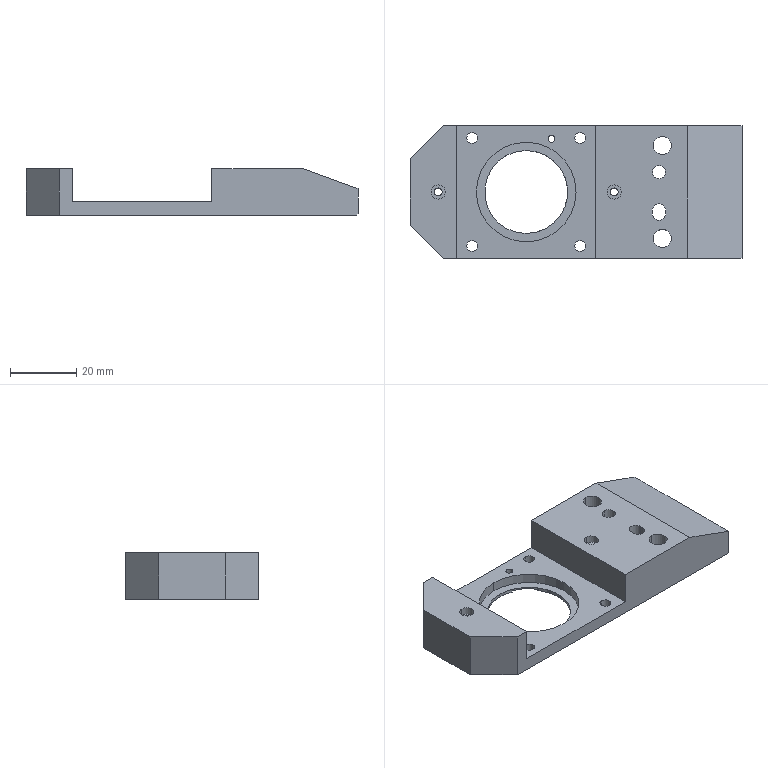NC program | NX | posted with a generic post | part box 100 x 40 x 14 mm
Lines 19 to 1361 of 15435:
(ADAPTIVE_MILLING_COPY , TOOL : D10)
N36 T04 M6
N38 G54
N40 G17 G0 G90 X-60.658 Y-0.012 S4000 M3
N42 G43 Z30. H4
N44 Z-13.
N46 G94 G1 Z-14. F1000.
N48 X-59.988 Y-0.372 F2200.
N50 X-59.306 Y-0.709
N52 G3 X-58.012 Y-0.012 R1.014
N54 X-57.807 Y4.262 R25.796
N56 G1 X-57.804 Y5.087
N58 X-57.802 Y6.337
N60 X-57.801 Y8.662
N62 X-57.8 Y21.587
N64 Y21.687
N66 X-57.797 Y21.787
N68 G2 X-54.247 Y26.731 R5.868
N70 X-49.332 Y27.731 R12.663
N72 X-41.858 Y27.797 R436.949
N74 G1 X-17.558
N76 X51.642
N78 X51.742 Y27.795
N80 X51.842 Y27.791
N82 X51.917 Y27.787
N84 X51.992 Y27.782
N86 G2 X56.775 Y24.149 R5.928
N88 X57.741 Y19.049 R13.335
N90 X57.796 Y11.775 R571.146
N92 G1 Y-21.6
N94 X57.795 Y-21.7
N96 X57.793 Y-21.775
N98 X57.79 Y-21.85
N100 X57.784 Y-21.95
N102 X57.778 Y-22.025
N104 G2 X54.072 Y-26.81 R5.956
N106 X49.165 Y-27.738 R13.286
N108 X37.666 Y-27.797 R661.267
N110 G1 X-51.634
N112 X-51.734 Y-27.795
N114 X-51.834 Y-27.792
N116 X-51.909 Y-27.787
N118 X-51.984 Y-27.782
N120 X-52.084 Y-27.773
N122 G2 X-56.813 Y-24.064 R5.968
N124 X-57.741 Y-19.031 R13.527
N126 X-57.764 Y-0.657 R809.741
N128 G3 X-57.604 Y8.715 R170.554
N130 G2 X-57.575 Y20.839 R747.675
N132 X-53.065 Y26.591 R6.941
N134 X-47.75 Y27.529 R15.579
N136 X-38.776 Y27.595 R512.073
N138 G1 X-9.076
N140 X-8.226 Y27.596
N142 X-7.826
N144 X-7.476
N146 X-7.201
N148 X-6.801 Y27.597
N150 X-5.826
N152 X-4.526
N154 X-4.051
N156 X-3.701
N158 X-3.376
N160 X-3.026
N162 X-2.701
N164 X-2.351
N166 X-2.026
N168 X-1.676
N170 X-1.351
N172 X-1.001
N174 X-0.651
N176 X-0.326
N178 X0.599
N180 X1.524
N182 X2.699
N184 X3.499
N186 X4.974
N188 X5.399
N190 X6.424
N192 X7.224
N194 X7.874
N196 X9.024
N198 X9.849
N200 X10.749
N202 X12.074
N204 X12.399
N206 X12.824
N208 X13.449
N210 X14.049
N212 X14.674
N214 X15.274
N216 X15.899
N218 X17.099
N220 X17.924
N222 X18.249
N224 X18.674
N226 X21.174
N228 X22.599
N230 X23.749
N232 X24.399
N234 X25.024
N236 X25.824
N238 X27.249 Y27.598
N240 X27.924 Y27.597
N242 X28.724
N244 X29.124
N246 X30.474
N248 X31.174
N250 X31.474
N252 X31.799
N254 X32.099
N256 X32.924
N258 X33.224
N260 X33.524
N262 X33.849
N264 X34.199
N266 X34.499
N268 X35.324
N270 X35.649
N272 X36.074
N274 X36.699
N276 X37.899
N278 X38.724
N280 X39.049
N282 X39.474
N284 X40.799 Y27.598
N286 X41.874 Y27.597
N288 X43.199
N290 X43.524
N292 X43.849
N294 X44.174
N296 X45.274 Y27.598
N298 X45.599 Y27.597
N300 X46.424
N302 X46.774
N304 X47.124
N306 X47.449
N308 X47.799
N310 X48.149
N312 X48.499
N314 X48.824
N316 X49.174
N318 X49.524
N320 X49.874
N322 X50.249
N324 X50.374 Y27.595
N326 X50.474 Y27.593
N328 X50.549 Y27.59
N330 X50.649 Y27.584
N332 X50.723 Y27.579
N334 X50.823 Y27.572
N336 G2 X56.565 Y23.122 R6.923
N338 X57.528 Y17.737 R15.471
N340 X57.594 Y8.263 R533.615
N342 G1 Y-20.262
N344 X57.593 Y-20.362
N346 X57.59 Y-20.462
N348 X57.586 Y-20.562
N350 X57.581 Y-20.662
N352 X57.574 Y-20.762
N354 G2 X53.061 Y-26.59 R6.93
N356 X47.671 Y-27.531 R15.729
N358 X37.197 Y-27.595 R619.863
N360 G1 X-50.253
N362 X-50.378 Y-27.593
N364 X-50.478 Y-27.59
N366 X-50.578 Y-27.586
N368 X-50.678 Y-27.581
N370 X-50.777 Y-27.573
N372 G2 X-56.576 Y-23.093 R6.924
N374 X-57.534 Y-17.556 R15.875
N376 X-57.552 Y-0.857 R593.714
N378 G3 X-57.405 Y10.841 R287.782
N380 G2 X-57.367 Y19.915 R332.032
N382 X-52.272 Y26.382 R7.62
N384 X-46.402 Y27.333 R17.997
N386 X-31.028 Y27.393 R794.051
N388 G1 X-10.478
N390 X-10.153 Y27.394
N392 X-9.853
N394 X-9.478 Y27.395
N396 X-8.753
N398 X-8.178
N400 X-7.628 Y27.396
N402 X-7.278
N404 X-6.928
N406 X-6.128
N408 X-5.353 Y27.397
N410 X-5.028
N412 X-4.603
N414 X-4.053
N416 X-3.553
N418 X-2.953
N420 X-2.653
N422 X-2.353
N424 X-1.978
N426 X-1.578
N428 X-0.778
N430 X-0.078
N432 X1.297
N434 X2.897 Y27.398
N436 X3.547 Y27.397
N438 X4.022
N440 X4.322
N442 X4.622
N444 X6.547
N446 X7.422
N448 X7.972
N450 X8.497
N452 X8.822
N454 X9.197
N456 X10.197
N458 X11.222
N460 X12.047
N462 X12.722
N464 X13.272
N466 X14.072
N468 X14.397
N470 X15.397
N472 X16.172
N474 X16.672
N476 X17.272
N478 X18.372
N480 X18.722
N482 X19.672
N484 X19.997
N486 X20.397
N488 X21.047
N490 X21.472
N492 X21.872
N494 X22.647
N496 X23.047
N498 X23.622
N500 X25.147
N502 X26.472
N504 X27.022
N506 X27.347
N508 X27.672
N510 X27.972
N512 X28.347
N514 X30.472
N516 X31.297
N518 X32.322
N520 X32.822
N522 X33.222
N524 X34.022
N526 X34.422
N528 X34.947
N530 G2 X49.871 Y27.364 R852.398
N532 X56.365 Y22.307 R7.605
N534 X57.328 Y16.49 R17.652
N536 X57.392 Y6.341 R626.425
N538 G1 Y-19.034
N540 X57.391 Y-19.184
N542 X57.388 Y-19.309
N544 X57.384 Y-19.459
N546 X57.379 Y-19.584
N548 X57.372 Y-19.709
N550 G2 X52.293 Y-26.371 R7.602
N552 X46.5 Y-27.328 R17.677
N554 X35.426 Y-27.393 R648.625
N556 G1 X-49.024
N558 X-49.199 Y-27.391
N560 X-49.349 Y-27.388
N562 X-49.474 Y-27.384
N564 X-49.599 Y-27.379
N566 X-49.724 Y-27.371
N568 G2 X-56.366 Y-22.303 R7.598
N570 X-57.32 Y-16.685 R17.277
N572 X-57.224 Y4.487 R468.954
N574 X-57.172 Y18.961 R932.099
N576 X-51.572 Y26.18 R8.162
N578 X-45.672 Y27.121 R19.16
N580 X-28.373 Y27.191 R845.532
N582 G1 X-11.873
N584 X-11.498 Y27.192
N586 X-11.123
N588 X-10.723 Y27.193
N590 X-10.273
N592 X-9.948 Y27.194
N594 X-9.548
N596 X-8.973 Y27.195
N598 X-8.648
N600 X-8.298
N602 X-7.998
N604 X-7.173 Y27.196
N606 X-6.773
N608 X-5.948
N610 X-5.423 Y27.197
N612 X-4.473
N614 X-3.023
N616 X-2.748
N618 X-2.473
N620 X-2.173
N622 X-1.798
N624 X-1.248
N626 X-0.373
N628 X0.977 Y27.198
N630 X1.252 Y27.197
N632 X1.552 Y27.198
N634 X2.377 Y27.197
N636 X2.802 Y27.198
N638 X3.402
N640 X4.552
N642 X5.002 Y27.197
N644 X5.377
N646 X5.677
N648 X6.677
N650 X7.152
N652 X7.477
N654 X7.877
N656 X8.627
N658 X8.927
N660 X9.627
N662 X10.152
N664 X10.452
N666 X11.302
N668 X11.977
N670 X12.477
N672 X13.327
N674 X13.652 Y27.198
N676 X14.027 Y27.197
N678 X14.552
N680 X15.052 Y27.198
N682 X17.102 Y27.197
N684 X17.677
N686 X17.977
N688 X18.327
N690 X18.627
N692 X18.927
N694 X19.302
N696 X19.627
N698 X20.727
N700 X21.402
N702 X22.027
N704 X22.627
N706 X23.702
N708 X24.102
N710 X24.852
N712 X25.877 Y27.198
N714 X26.677 Y27.197
N716 X27.202
N718 X27.527
N720 X28.652
N722 X29.952
N724 X30.552
N726 X30.852
N728 X31.427
N730 X32.277
N732 X32.652
N734 X32.977
N736 X33.252
N738 X33.552
N740 X33.927
N742 X34.177
N744 X34.502
N746 X34.852
N748 X35.777
N750 X36.627
N752 X36.977
N754 X37.277
N756 X37.702
N758 G2 X49.002 Y27.161 R605.97
N760 X56.159 Y21.621 R8.144
N762 X57.122 Y15.575 R19.209
N764 X57.19 Y5.55 R621.552
N766 G1 Y-17.95
N768 X57.188 Y-18.15
N770 X57.186 Y-18.325
N772 X57.182 Y-18.5
N774 X57.176 Y-18.649
N776 X57.169 Y-18.799
N778 G2 X51.667 Y-26.142 R8.138
N780 X45.649 Y-27.12 R18.936
N782 X29.05 Y-27.191 R817.893
N784 G1 X-8.375
N786 X-9.225 Y-27.192
N788 X-9.625
N790 X-10.1
N792 X-10.525
N794 X-10.875
N796 X-11.2 Y-27.193
N798 X-12.125
N800 X-12.975
N802 X-13.275
N804 X-13.575
N806 X-15.125
N808 X-15.825
N810 X-17.
N812 X-17.7
N814 X-18.875
N816 X-19.425
N818 X-19.775
N820 X-20.1
N822 X-21.2
N824 X-21.525
N826 X-21.85
N828 X-22.675
N830 X-23.65
N832 X-24.275
N834 X-25.6
N836 X-26.2
N838 X-26.525
N840 X-26.825
N842 X-27.65
N844 X-28.45
N846 X-29.625
N848 X-30.275
N850 X-30.875
N852 X-31.5
N854 X-32.1
N856 X-32.725
N858 X-33.325
N860 X-33.95
N862 X-34.55
N864 X-35.175
N866 X-35.775
N868 X-36.4
N870 X-37.
N872 X-37.625
N874 X-38.225
N876 X-38.85
N878 X-39.45
N880 X-40.075
N882 X-40.675
N884 X-41.3
N886 G2 X-49.174 Y-27.144 R190.539
N888 X-56.123 Y-21.714 R8.121
N890 X-57.115 Y-15.774 R18.568
N892 X-57.026 Y4.774 R495.094
N894 X-56.966 Y18.248 R708.359
N896 X-51.062 Y25.935 R8.596
N898 X-44.966 Y26.912 R20.074
N900 X-33.916 Y26.989 R534.348
N902 G1 X-13.291
N904 X-12.891 Y26.99
N906 X-12.591
N908 X-12.166 Y26.991
N910 X-11.216 Y26.992
N912 X-10.566 Y26.993
N914 X-10.016
N916 X-9.216 Y26.994
N918 X-8.366 Y26.995
N920 X-7.216 Y26.996
N922 X-6.666
N924 X-6.266
N926 X-5.816
N928 X-4.516
N930 X-3.716 Y26.997
N932 X-2.866
N934 X-2.566
N936 X-2.291
N938 X-1.966
N940 X-1.641
N942 X-0.741
N944 X-0.116
N946 X0.309
N948 X1.109
N950 X2.034
N952 X2.609
N954 X3.209 Y26.998
N956 X3.609 Y26.997
N958 X4.009 Y26.998
N960 X4.309 Y26.997
N962 X4.684
N964 X5.234
N966 X5.534
N968 X6.159
N970 X6.959
N972 X7.359
N974 X7.959
N976 X8.484
N978 X8.834
N980 X10.234
N982 X10.534
N984 X10.834
N986 X11.734
N988 X12.259
N990 X12.609
N992 X13.009
N994 X13.309
N996 X13.709 Y26.998
N998 X14.659 Y26.997
N1000 X16.384
N1002 X16.684
N1004 X16.984
N1006 X17.409
N1008 X18.084
N1010 X19.709
N1012 X20.634
N1014 X21.259
N1016 X21.784
N1018 X22.709
N1020 X23.859
N1022 X24.434 Y26.998
N1024 X24.909 Y26.997
N1026 X26.509
N1028 X27.409
N1030 X28.659
N1032 X29.509
N1034 X29.884
N1036 X30.459
N1038 X30.959
N1040 X31.259
N1042 X31.609
N1044 X32.009
N1046 X32.534
N1048 X32.909
N1050 X33.184
N1052 X33.484
N1054 X34.359
N1056 G2 X48.233 Y26.958 R698.776
N1058 X55.939 Y21.045 R8.594
N1060 X56.913 Y14.873 R20.196
N1062 X56.988 Y1.748 R627.827
N1064 G1 Y-16.977
N1066 X56.987 Y-17.152
N1068 X56.985 Y-17.352
N1070 X56.982 Y-17.527
N1072 X56.977 Y-17.702
N1074 X56.971 Y-17.877
N1076 G2 X50.93 Y-25.98 R8.63
N1078 X44.576 Y-26.924 R21.193
N1080 X33.476 Y-26.989 R651.446
N1082 G1 X-6.974
N1084 X-7.299 Y-26.99
N1086 X-7.599
N1088 X-7.974
N1090 X-8.874 Y-26.991
N1092 X-9.174
N1094 X-9.549
N1096 X-10.124 Y-26.992
N1098 X-10.424
N1100 X-10.799
N1102 X-11.349
N1104 X-11.674
N1106 X-12.224 Y-26.993
N1108 X-12.524 Y-26.992
N1110 X-13.474 Y-26.993
N1112 X-13.749
N1114 X-15.549
N1116 X-16.799
N1118 X-18.199
N1120 X-20.524
N1122 X-21.074
N1124 X-21.924
N1126 X-22.499
N1128 X-22.799
N1130 X-23.349
N1132 X-23.699
N1134 X-24.574
N1136 X-24.874
N1138 X-25.174
N1140 X-25.599
N1142 X-26.074
N1144 X-26.849
N1146 X-27.124
N1148 X-27.399
N1150 X-27.699
N1152 X-28.674
N1154 X-29.524
N1156 X-30.074
N1158 X-30.924
N1160 X-31.249
N1162 X-31.674
N1164 X-32.274
N1166 X-32.824
N1168 X-33.524
N1170 X-33.974
N1172 X-34.274
N1174 X-34.624
N1176 X-35.074
N1178 X-35.599
N1180 X-36.274
N1182 X-36.749
N1184 X-37.049
N1186 X-37.349
N1188 X-38.249
N1190 X-38.624
N1192 X-39.349
N1194 X-39.824
N1196 X-40.124
N1198 X-40.499
N1200 X-41.349
N1202 X-41.649
N1204 G2 X-48.597 Y-26.924 R116.253
N1206 X-55.944 Y-21.028 R8.585
N1208 X-56.92 Y-14.705 R20.626
N1210 X-56.826 Y5.168 R529.552
N1212 X-56.764 Y17.542 R590.002
N1214 X-50.503 Y25.728 R8.999
N1216 X-44.004 Y26.715 R21.688
N1218 X-34.404 Y26.786 R610.822
N1220 G1 X-20.479 Y26.787
N1222 X-14.704
N1224 X-14.279 Y26.788
N1226 X-13.979
N1228 X-13.629 Y26.789
N1230 X-13.304
N1232 X-12.929
N1234 X-12.304 Y26.79
N1236 X-11.604 Y26.791
N1238 X-9.829 Y26.794
N1240 X-8.904
N1242 X-8.504
N1244 X-8.004 Y26.795
N1246 X-7.204
N1248 X-6.879
N1250 X-6.054 Y26.796
N1252 X-4.879 Y26.797
N1254 X-4.554
N1256 X-3.929
N1258 X-3.529
N1260 X-2.904
N1262 X-2.429
N1264 X-1.554
N1266 X-1.179
N1268 X-0.879
N1270 X0.121
N1272 X0.946
N1274 X1.246
N1276 X1.871 Y26.798
N1278 X2.221 Y26.797
N1280 X2.621 Y26.798
N1282 X2.921 Y26.797
N1284 X3.321
N1286 X3.596
N1288 X3.971
N1290 X4.471
N1292 X4.771
N1294 X5.071
N1296 X5.371
N1298 X5.921
N1300 X6.221
N1302 X6.921
N1304 X7.446
N1306 X8.421
N1308 X9.246
N1310 X9.521
N1312 X9.821
N1314 X10.796
N1316 X11.746
N1318 X12.296
N1320 X12.596
N1322 X12.921
N1324 X13.296
N1326 X13.821
N1328 X14.696
N1330 X15.046
N1332 X15.746
N1334 X16.246
N1336 X16.571
N1338 X16.946
N1340 X17.246
N1342 X17.571
N1344 X19.021
N1346 X20.196
N1348 X21.646
N1350 X21.946
N1352 X22.771
N1354 X23.071
N1356 X23.396
N1358 X23.746
N1360 X24.146
N1362 X25.471
N1364 X26.321
N1366 X27.496
N1368 X27.821
N1370 X28.221
N1372 X28.696
N1374 X28.996
N1376 X29.346
N1378 X29.771
N1380 X30.396
N1382 X30.971
N1384 X31.521
N1386 X31.871
N1388 X32.421
N1390 G2 X47.47 Y26.759 R837.178
N1392 X55.746 Y20.445 R9.005
N1394 X56.71 Y14.067 R21.68
N1396 X56.786 Y0.243 R684.127
N1398 G1 X56.785 Y-16.107
N1400 X56.784 Y-16.357
N1402 X56.782 Y-16.582
N1404 X56.778 Y-16.807
N1406 X56.773 Y-16.982
N1408 X56.766 Y-17.182
N1410 G2 X50.477 Y-25.734 R9.013
N1412 X44.301 Y-26.702 R21.031
N1414 X34.077 Y-26.786 R443.88
N1416 G1 X16.577 Y-26.787
N1418 X-5.573
N1420 X-5.923 Y-26.788
N1422 X-6.223
N1424 X-6.573 Y-26.789
N1426 X-6.898
N1428 X-7.223
N1430 X-7.548
N1432 X-7.973 Y-26.79
N1434 X-8.548
N1436 X-9.423 Y-26.791
N1438 X-10.223
N1440 X-10.523
N1442 X-10.923 Y-26.792
N1444 X-11.748
N1446 X-12.098
N1448 X-12.398
N1450 X-12.698
N1452 X-13.523 Y-26.793
N1454 X-14.848
N1456 X-16.323
N1458 X-17.098
N1460 X-17.398
N1462 X-17.698
N1464 X-18.723
N1466 X-20.298
N1468 X-21.123
N1470 X-21.498
N1472 X-22.073
N1474 X-23.173
N1476 X-23.648
N1478 X-24.448
N1480 X-25.548
N1482 X-25.823
N1484 X-26.123
N1486 X-26.448
N1488 X-27.048
N1490 X-27.898
N1492 X-28.423
N1494 X-28.723
N1496 X-29.573
N1498 X-29.998
N1500 X-30.873
N1502 X-31.123
N1504 X-31.423
N1506 X-31.848
N1508 X-32.423
N1510 X-33.073
N1512 X-33.548
N1514 X-33.898
N1516 X-34.198
N1518 X-34.548
N1520 X-35.398
N1522 X-35.773
N1524 X-36.623
N1526 X-36.898
N1528 X-37.223
N1530 X-37.648
N1532 X-38.248
N1534 X-38.823
N1536 X-40.048
N1538 G2 X-47.797 Y-26.731 R166.798
N1540 X-55.721 Y-20.51 R8.973
N1542 X-56.713 Y-14.012 R21.589
N1544 X-56.631 Y5.186 R521.074
N1546 X-56.557 Y16.96 R462.345
N1548 X-50.06 Y25.493 R9.334
N1550 X-43.538 Y26.503 R22.039
N1552 X-32.864 Y26.584 R503.238
N1554 G1 X-16.114 Y26.585
N1556 X-15.689 Y26.586
N1558 X-15.339
N1560 X-15.014 Y26.587
N1562 X-14.714
N1564 X-14.314
N1566 X-13.739 Y26.588
N1568 X-13.464 Y26.589
N1570 X-13.139
N1572 X-12.764 Y26.59
N1574 X-12.464
N1576 X-12.164
N1578 X-11.314 Y26.592
N1580 X-10.789
N1582 X-10.139 Y26.593
N1584 X-9.239
N1586 X-8.114 Y26.594
N1588 X-6.614 Y26.595
N1590 X-6.264 Y26.596
N1592 X-5.939
N1594 X-5.539
N1596 X-4.914
N1598 X-4.289
N1600 X-3.789
N1602 X-3.514
N1604 X-3.189 Y26.597
N1606 X-2.814
N1608 X-2.564
N1610 X-2.264
N1612 X-1.889
N1614 X-1.439
N1616 X-0.964
N1618 X-0.589
N1620 X0.361 Y26.598
N1622 X0.886 Y26.597
N1624 X1.161 Y26.598
N1626 X1.536 Y26.597
N1628 X1.886
N1630 X2.236
N1632 X2.536
N1634 X2.911
N1636 X3.461
N1638 X3.836
N1640 X4.311
N1642 X4.636
N1644 X5.186
N1646 X5.511
N1648 X6.161
N1650 X6.686
N1652 X6.986
N1654 X7.286
N1656 X7.661
N1658 X8.586
N1660 X9.036
N1662 X9.936
N1664 X10.311
N1666 X10.636
N1668 X11.011
N1670 X11.286
N1672 X11.661
N1674 X12.586
N1676 X13.136
N1678 X13.686
N1680 X14.636
N1682 X15.211
N1684 X15.561
N1686 X15.911
N1688 X16.261
N1690 X16.811
N1692 X17.636
N1694 X18.461
N1696 X19.061
N1698 X19.361
N1700 X19.786
N1702 X20.286
N1704 X21.736
N1706 X22.136
N1708 X22.536
N1710 X23.411
N1712 X23.911
N1714 X24.961
N1716 X25.711
N1718 X26.061
N1720 X26.436
N1722 X27.411
N1724 X28.111
N1726 X28.611
N1728 X29.411
N1730 X29.836
N1732 X30.186
N1734 X30.536
N1736 X31.636
N1738 X31.961
N1740 X32.261
N1742 X32.661
N1744 X33.011
N1746 X33.361
N1748 X33.761
N1750 G2 X46.81 Y26.556 R730.966
N1752 X52.574 Y24.458 R10.133
N1754 X54.967 Y21.571 R6.003
N1756 X56.447 Y14.67 R19.016
N1758 X56.583 Y1.547 R295.283
N1760 G1 Y-15.278
N1762 X56.581 Y-15.628
N1764 X56.579 Y-15.878
N1766 X56.574 Y-16.103
N1768 X56.57 Y-16.278
N1770 X56.563 Y-16.478
N1772 G2 X54.473 Y-22.544 R9.936
N1774 X51.707 Y-24.904 R5.891
N1776 X44.57 Y-26.454 R18.988
N1778 X33.347 Y-26.584 R261.966
N1780 G1 X21.222
N1782 X-4.178 Y-26.585
N1784 X-4.553
N1786 X-4.953 Y-26.586
N1788 X-5.353 Y-26.587
N1790 X-5.853
N1792 X-6.203 Y-26.588
N1794 X-6.853
N1796 X-7.178 Y-26.589
N1798 X-7.478
N1800 X-7.778
N1802 X-8.103
N1804 X-8.503 Y-26.59
N1806 X-9.228
N1808 X-9.528 Y-26.591
N1810 X-9.828
N1812 X-10.228
N1814 X-10.728
N1816 X-11.028
N1818 X-11.403 Y-26.592
N1820 X-11.903
N1822 X-12.378
N1824 X-13.128
N1826 X-13.453
N1828 X-15.028 Y-26.593
N1830 X-15.878
N1832 X-16.353
N1834 X-17.403
N1836 X-18.578
N1838 X-19.528
N1840 X-20.478
N1842 X-21.128
N1844 X-21.928
N1846 X-22.278
N1848 X-22.578
N1850 X-23.478
N1852 X-24.503
N1854 X-24.878
N1856 X-25.503
N1858 X-26.053
N1860 X-26.828
N1862 X-27.128
N1864 X-28.503
N1866 X-28.853
N1868 X-29.228
N1870 X-29.828
N1872 X-30.453
N1874 X-31.553
N1876 X-31.853
N1878 X-32.203
N1880 X-32.578
N1882 X-32.953
N1884 X-33.453
N1886 X-33.753
N1888 X-34.153
N1890 G2 X-46.952 Y-26.543 R476.425
N1892 X-55.499 Y-20.032 R9.33
N1894 X-56.499 Y-13.584 R21.999
N1896 X-56.437 Y5.039 R464.728
N1898 X-56.351 Y16.413 R392.844
N1900 X-49.577 Y25.283 R9.651
N1902 X-43.004 Y26.295 R22.831
N1904 X-28.18 Y26.382 R605.401
N1906 G1 X-17.53
N1908 X-17.08 Y26.384
N1910 X-16.705
N1912 X-16.38 Y26.385
N1914 X-16.08
N1916 X-15.68
N1918 X-15.405 Y26.386
N1920 X-15.105
N1922 X-14.805 Y26.387
N1924 X-14.405
N1926 X-13.58 Y26.388
N1928 X-13.18 Y26.389
N1930 X-12.58 Y26.39
N1932 X-12.18
N1934 X-11.205 Y26.392
N1936 X-10.655
N1938 X-10.305 Y26.393
N1940 X-9.705
N1942 X-8.93 Y26.394
N1944 X-8.605
N1946 X-8.28
N1948 X-7.805 Y26.395
N1950 X-7.305
N1952 X-6.93
N1954 X-6.305
N1956 X-5.405 Y26.396
N1958 X-4.805
N1960 X-4.255
N1962 X-3.855
N1964 X-2.955
N1966 X-2.63 Y26.397
N1968 X-2.28 Y26.396
N1970 X-1.955 Y26.397
N1972 X-1.68
N1974 X-0.855
N1976 X-0.505
N1978 X0.145
N1980 X0.52
N1982 X0.845
N1984 X1.145
N1986 X1.445
N1988 X1.82
N1990 X3.07
N1992 X3.62
N1994 X4.12
N1996 X4.42
N1998 X5.02
N2000 X5.395
N2002 X6.045
N2004 X6.845
N2006 X7.145 Y26.398
N2008 X7.495 Y26.397
N2010 X8.27
N2012 X8.57
N2014 X8.92
N2016 X9.27
N2018 X10.195
N2020 X10.62
N2022 X11.145
N2024 X12.07
N2026 X12.945
N2028 X13.82
N2030 X14.195
N2032 X14.52
N2034 X14.87
N2036 X15.995
N2038 X16.27
N2040 X16.595
N2042 X16.895
N2044 X17.17
N2046 X17.995
N2048 X18.32
N2050 X18.645
N2052 X18.945
N2054 X19.795
N2056 X20.645
N2058 X20.995
N2060 X21.445
N2062 X21.945
N2064 X22.27
N2066 X22.67
N2068 X24.17
N2070 X24.67 Y26.398
N2072 X25.045 Y26.397
N2074 X25.545
N2076 X26.095 Y26.398
N2078 X26.495 Y26.397
N2080 X26.945
N2082 X27.245
N2084 X28.145
N2086 X28.495
N2088 X28.795
N2090 X29.12
N2092 X29.47
N2094 X29.745
N2096 X30.045
N2098 X30.345
N2100 X30.72
N2102 X31.295
N2104 X31.62
N2106 X32.02
N2108 X32.42
N2110 X33.695
N2112 X34.595
N2114 X35.07
N2116 X35.47
N2118 X36.52
N2120 X36.92
N2122 G2 X46.419 Y26.339 R271.025
N2124 X51.121 Y25.01 R11.956
N2126 X52.541 Y24.474 R7.89
N2128 G1 X53.109 Y24.055
N2130 X53.662 Y23.615
N2132 X54.458 Y22.574
N2134 G2 X56.13 Y15.686 R21.172
N2136 X56.379 Y5.143 R127.942
N2138 G1 X56.381 Y2.443
N2140 Y-8.557
N2142 Y-14.507
N2144 X56.379 Y-14.857
N2146 X56.376 Y-15.182
N2148 X56.371 Y-15.432
N2150 G2 X55.011 Y-21.111 R12.182
N2152 X54.483 Y-22.518 R7.214
N2154 G3 X56.6 Y-22.953 R-1.1
N2156 G1 X57.151 Y21.533
N2158 G3 X54.972 Y21.332 R-1.1
N2160 G2 X55.809 Y16.473 R138.57
N2162 X56.173 Y6.76 R87.644
N2164 G1 X56.176 Y5.385
N2166 X56.178 Y3.285
N2168 X56.179 Y-0.99
N2170 Y-13.765
N2172 X56.177 Y-14.115
N2174 X56.173 Y-14.515
N2176 G2 X55.121 Y-20.219 R15.36
N2178 G1 X54.994 Y-21.185
N2180 G3 X57.185 Y-21.33 R-1.1
N2182 G1 X57.209 Y21.146
N2184 G3 X55.018 Y21.003 R-1.1
N2186 G2 X55.821 Y13.705 R120.972
N2188 X55.976 Y1.707 R263.089
N2190 X55.935 Y-15.042 R900.75
N2192 X55.152 Y-19.412 R21.367
N2194 G1 X55.15 Y-19.438
N2196 Y-19.967
N2198 X55.146 Y-20.033
N2200 X55.12 Y-20.231
N2202 G3 X57.31 Y-20.376 R-1.1
N2204 G1 X57.35 Y19.966
N2206 G3 X56.249 Y21.065 R1.1
N2208 X55.15 Y19.967 R1.1
N2210 X55.503 Y15.208 R52.7
N2212 G2 X55.772 Y3.539 R160.389
N2214 G1 X55.774 Y1.039
N2216 X55.775 Y-4.911
N2218 Y-12.386
N2220 X55.772 Y-12.836
N2222 X55.769 Y-13.236
N2224 X55.764 Y-13.536
N2226 G2 X55.15 Y-18.488 R24.182
N2228 G1 Y-19.438
N2230 G3 X56.252 Y-20.536 R1.1
N2232 X57.35 Y-19.438 R1.1
N2234 G1 Y19.367
N2236 G3 X56.248 Y20.465 R1.1
N2238 X55.15 Y19.367 R1.1
N2240 X55.405 Y13.499 R77.246
N2242 G2 X55.572 Y0.452 R300.541
N2244 X55.521 Y-14.147 R594.252
N2246 X55.15 Y-17.256 R37.271
N2248 G1 Y-18.506
N2250 G3 X56.252 Y-19.604 R1.1
N2252 X57.35 Y-18.506 R1.1
N2254 G1 Y17.967
N2256 G3 X56.248 Y19.065 R1.1
N2258 X55.15 Y17.967 R1.1
N2260 X55.329 Y9.245 R285.488
N2262 G1 X55.339 Y8.495
N2264 X55.346 Y7.745
N2266 X55.353 Y6.97
N2268 X55.358 Y5.97
N2270 X55.363 Y4.845
N2272 X55.366 Y3.395
N2274 X55.369 Y1.395
N2276 X55.37 Y-1.955
N2278 G2 X55.305 Y-13.904 R350.037
N2280 G3 X55.15 Y-17.28 R24.41
N2282 X56.252 Y-18.378 R1.1
N2284 X57.35 Y-17.28 R1.1
N2286 G1 Y15.542
N2288 G3 X56.248 Y16.64 R1.1
N2290 X55.15 Y15.542 R1.1
N2292 G1 Y5.467
N2294 X55.154 Y5.017
N2296 X55.159 Y4.192
N2298 X55.163 Y3.117
N2300 X55.166 Y1.617
N2302 X55.167 Y-0.733
N2304 X55.168 Y-5.908
N2306 Y-10.533
N2308 X55.166 Y-11.058
N2310 X55.161 Y-11.583
N2312 X55.157 Y-11.883
N2314 X55.151 Y-12.183
N2316 X55.15 Y-12.22
N2318 Y-15.62
N2320 G3 X56.252 Y-16.718 R1.1
N2322 X57.35 Y-15.62 R1.1
N2324 G1 Y5.467
N2326 G3 X56.248 Y6.565 R1.1
N2328 X55.15 Y5.467 R1.1
N2330 G1 Y-12.233
N2332 X55.146 Y-20.033
N2334 X54.962 Y-21.364
N2336 X54.44 Y-22.601
N2338 X53.615 Y-23.662
N2340 X52.574 Y-24.458
N2342 G2 X45.761 Y-26.123 R21.139
N2344 X36.093 Y-26.379 R113.682
N2346 G1 X34.093 Y-26.381
N2348 X29.968 Y-26.382
N2350 X-2.757
N2352 X-3.157 Y-26.383
N2354 X-3.482 Y-26.384
N2356 X-3.857
N2358 X-4.157 Y-26.385
N2360 X-4.482
N2362 X-4.807 Y-26.386
N2364 X-5.107
N2366 X-5.482
N2368 X-6.182 Y-26.387
N2370 X-6.882 Y-26.388
N2372 X-7.982 Y-26.389
N2374 X-8.457
N2376 X-8.807 Y-26.39
N2378 X-9.382 Y-26.391
N2380 X-9.732
N2382 X-10.257
N2384 X-10.582
N2386 X-10.882
N2388 X-11.657 Y-26.392
N2390 X-12.457
N2392 X-13.532 Y-26.393
N2394 X-13.882 Y-26.392
N2396 X-14.707 Y-26.393
N2398 X-15.057
N2400 X-16.357
N2402 X-18.357
N2404 X-19.082
N2406 X-19.457
N2408 X-20.382
N2410 X-20.932
N2412 X-21.282
N2414 X-22.182
N2416 X-22.657
N2418 X-23.832
N2420 X-24.407
N2422 X-24.932
N2424 X-25.982
N2426 X-27.907
N2428 X-28.832
N2430 X-29.357
N2432 X-30.257
N2434 X-31.007
N2436 X-31.632
N2438 X-32.232
N2440 X-32.807
N2442 G2 X-46.232 Y-26.347 R643.477
N2444 X-55.313 Y-19.475 R9.674
N2446 X-56.298 Y-12.872 R23.371
N2448 X-56.241 Y4.726 R444.372
N2450 X-56.147 Y15.875 R361.321
N2452 X-49.146 Y25.063 R9.936
N2454 X-42.324 Y26.093 R23.796
N2456 X-27.224 Y26.18 R647.732
N2458 G1 X-18.924
N2460 X-18.449 Y26.182
N2462 X-17.599 Y26.183
N2464 X-17.149 Y26.184
N2466 X-16.749
N2468 X-16.474 Y26.185
N2470 X-16.149
N2472 X-15.549 Y26.186
N2474 X-15.224
N2476 X-14.799 Y26.187
N2478 X-14.324
N2480 X-14.024 Y26.188
N2482 X-13.674
N2484 X-13.324 Y26.189
N2486 X-12.849 Y26.19
N2488 X-12.049 Y26.191
N2490 X-11.724
N2492 X-11.374
N2494 X-11.099 Y26.192
N2496 X-10.774
N2498 X-10.149 Y26.193
N2500 X-9.624
N2502 X-9.249
N2504 X-8.249 Y26.194
N2506 X-7.674
N2508 X-6.849 Y26.195
N2510 X-6.499
N2512 X-5.899 Y26.196
N2514 X-5.599
N2516 X-4.299
N2518 X-3.999
N2520 X-3.649
N2522 X-3.299
N2524 X-2.449
N2526 X-1.524 Y26.197
N2528 X-1.224 Y26.196
N2530 X-0.874 Y26.197
N2532 X-0.499
N2534 X-0.124
N2536 X0.476
N2538 X1.851
N2540 X2.151
N2542 X2.551
N2544 X3.326
N2546 X3.626
N2548 X3.976
N2550 X4.276
N2552 X4.701
N2554 X5.226
N2556 X5.576
N2558 X6.426
N2560 X7.326
N2562 X7.601
N2564 X7.901
N2566 X8.201
N2568 X8.501
N2570 X8.826
N2572 X9.151
N2574 X9.501
N2576 X10.326
N2578 X10.626
N2580 X10.926
N2582 X11.276
N2584 X12.326
N2586 X13.151
N2588 X14.151
N2590 X15.051
N2592 X15.826
N2594 X16.126
N2596 X16.951
N2598 X17.276
N2600 X17.576
N2602 X17.876
N2604 X18.726
N2606 X19.376
N2608 X19.651
N2610 X19.951
N2612 X20.326
N2614 X20.626
N2616 X21.051
N2618 X22.101
N2620 X22.876
N2622 X23.301
N2624 X23.626
N2626 X23.976
N2628 X24.301
N2630 X24.726
N2632 X25.001
N2634 X25.301
N2636 X25.626
N2638 X26.051
N2640 X26.526
N2642 X26.876
N2644 X27.176
N2646 X27.751
N2648 X28.076
N2650 X28.426
N2652 X29.151
N2654 X29.601
N2656 X30.001
N2658 X30.251
N2660 G2 X45.65 Y26.148 R713.317
N2662 X50.246 Y25.118 R15.471
N2664 G1 X51.188 Y24.994
N2666 G3 X51.752 Y25.084 R1.052
N2668 G1 X52.473 Y25.43
N2670 X54.276 Y26.295 Z-13.9
N2672 G2 X55.535 Y26.158 R1.037
N2674 G1 X55.975 Y25.718
N2676 X56.38 Y25.246
N2678 X56.708 Y24.72
N2680 X57.284 Y23.615
N2682 X57.818 Y22.49
N2684 G2 X58.098 Y21.291 R3.666
N2686 G1 X58.367 Y16.39
N2688 X58.61 Y11.488
N2690 G2 X58.687 Y-2.425 R196.399
N2692 G1 X58.085 Y-22.198
N2694 G2 X56.857 Y-24.989 R4.096
N2696 G1 X56.217 Y-25.621
N2698 X55.561 Y-26.235
N2700 G2 X54.392 Y-26.246 R1.065
N2702 G1 X52.597 Y-25.364 Z-14.
N2704 X52.21 Y-25.173
N2706 X51.816 Y-24.996
N2708 X51.576 Y-24.958
N2710 X51.332 Y-24.972
N2712 G2 X46.349 Y-25.824 R123.58
N2714 X36.86 Y-26.174 R88.429